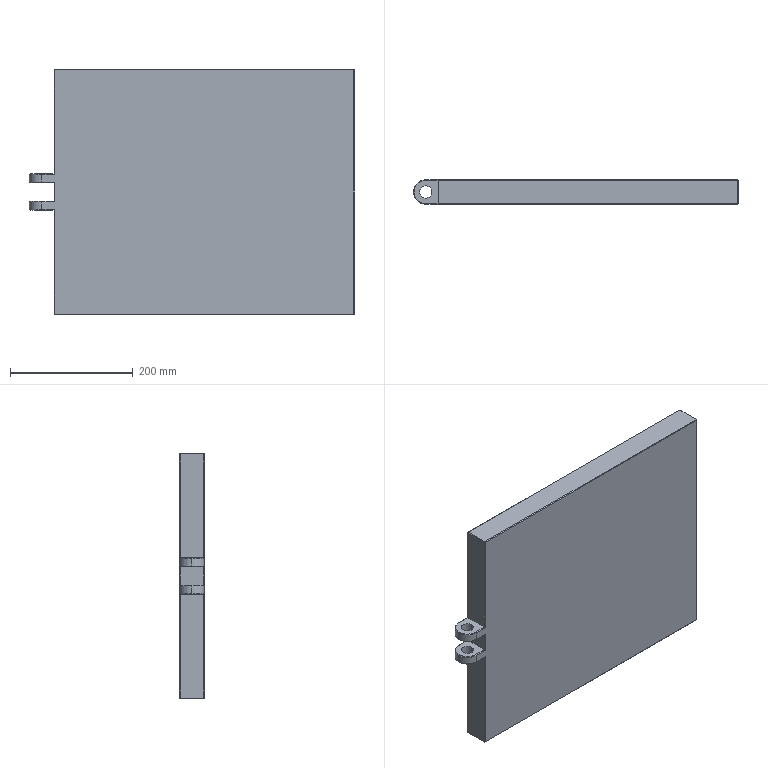Part | SolidWorks | 1 solid | 58 faces | box 530 x 40 x 400 mm | volume 7871394 mm3 | plane 44 | cylinder 8 | cone 6 | commonest cylinder face diameters 20 x4 40 x4
STEP:
#1=CARTESIAN_POINT('',(-284.,20.,30.));
#2=VERTEX_POINT('',#1);
#3=CARTESIAN_POINT('',(-265.,1.,30.));
#4=VERTEX_POINT('',#3);
#5=CARTESIAN_POINT('',(-265.,20.,30.));
#6=DIRECTION('',(0.,0.,1.));
#7=DIRECTION('',(1.,0.,0.));
#8=AXIS2_PLACEMENT_3D('',#5,#6,#7);
#9=CIRCLE('',#8,19.);
#10=EDGE_CURVE('',#2,#4,#9,.T.);
#11=ORIENTED_EDGE('',*,*,#10,.F.);
#12=CARTESIAN_POINT('',(-285.,20.,29.));
#13=VERTEX_POINT('',#12);
#14=CARTESIAN_POINT('',(-284.,20.,30.));
#15=DIRECTION('',(-0.7071,0.,-0.7071));
#16=VECTOR('',#15,1000.);
#17=LINE('',#14,#16);
#18=EDGE_CURVE('',#2,#13,#17,.T.);
#19=ORIENTED_EDGE('',*,*,#18,.T.);
#20=CARTESIAN_POINT('',(-265.,0.,29.));
#21=VERTEX_POINT('',#20);
#22=CARTESIAN_POINT('',(-265.,20.,29.));
#23=DIRECTION('',(0.,0.,-1.));
#24=DIRECTION('',(1.,0.,0.));
#25=AXIS2_PLACEMENT_3D('',#22,#23,#24);
#26=CIRCLE('',#25,20.);
#27=EDGE_CURVE('',#21,#13,#26,.T.);
#28=ORIENTED_EDGE('',*,*,#27,.F.);
#29=CARTESIAN_POINT('',(-265.,1.,30.));
#30=DIRECTION('',(0.,-0.7071,-0.7071));
#31=VECTOR('',#30,1000.);
#32=LINE('',#29,#31);
#33=EDGE_CURVE('',#4,#21,#32,.T.);
#34=ORIENTED_EDGE('',*,*,#33,.F.);
#35=EDGE_LOOP('',(#11,#19,#28,#34));
#36=FACE_OUTER_BOUND('',#35,.T.);
#37=CARTESIAN_POINT('',(-265.,20.,30.));
#38=DIRECTION('',(0.,0.,-1.));
#39=DIRECTION('',(-1.,0.,0.));
#40=AXIS2_PLACEMENT_3D('',#37,#38,#39);
#41=CONICAL_SURFACE('',#40,19.,0.7854);
#42=ADVANCED_FACE('',(#36),#41,.T.);
#43=CARTESIAN_POINT('',(-284.,20.,-15.));
#44=VERTEX_POINT('',#43);
#45=CARTESIAN_POINT('',(-265.,1.,-15.));
#46=VERTEX_POINT('',#45);
#47=CARTESIAN_POINT('',(-265.,20.,-15.));
#48=DIRECTION('',(0.,0.,1.));
#49=DIRECTION('',(-1.,0.,0.));
#50=AXIS2_PLACEMENT_3D('',#47,#48,#49);
#51=CIRCLE('',#50,19.);
#52=EDGE_CURVE('',#44,#46,#51,.T.);
#53=ORIENTED_EDGE('',*,*,#52,.F.);
#54=CARTESIAN_POINT('',(-285.,20.,-16.));
#55=VERTEX_POINT('',#54);
#56=CARTESIAN_POINT('',(-285.,20.,-16.));
#57=DIRECTION('',(-0.7071,0.,-0.7071));
#58=VECTOR('',#57,1000.);
#59=LINE('',#56,#58);
#60=EDGE_CURVE('',#44,#55,#59,.T.);
#61=ORIENTED_EDGE('',*,*,#60,.T.);
#62=CARTESIAN_POINT('',(-265.,0.,-16.));
#63=VERTEX_POINT('',#62);
#64=CARTESIAN_POINT('',(-265.,20.,-16.));
#65=DIRECTION('',(0.,0.,-1.));
#66=DIRECTION('',(-1.,0.,0.));
#67=AXIS2_PLACEMENT_3D('',#64,#65,#66);
#68=CIRCLE('',#67,20.);
#69=EDGE_CURVE('',#63,#55,#68,.T.);
#70=ORIENTED_EDGE('',*,*,#69,.F.);
#71=CARTESIAN_POINT('',(-265.,1.,-15.));
#72=DIRECTION('',(0.,-0.7071,-0.7071));
#73=VECTOR('',#72,1000.);
#74=LINE('',#71,#73);
#75=EDGE_CURVE('',#46,#63,#74,.T.);
#76=ORIENTED_EDGE('',*,*,#75,.F.);
#77=EDGE_LOOP('',(#53,#61,#70,#76));
#78=FACE_OUTER_BOUND('',#77,.T.);
#79=CARTESIAN_POINT('',(-265.,20.,-16.));
#80=DIRECTION('',(0.,0.,-1.));
#81=DIRECTION('',(-1.,0.,0.));
#82=AXIS2_PLACEMENT_3D('',#79,#80,#81);
#83=CONICAL_SURFACE('',#82,20.,0.7854);
#84=ADVANCED_FACE('',(#78),#83,.T.);
#85=CARTESIAN_POINT('',(-275.,20.,-30.));
#86=VERTEX_POINT('',#85);
#87=CARTESIAN_POINT('',(-255.,20.,-30.));
#88=VERTEX_POINT('',#87);
#89=CARTESIAN_POINT('',(-265.,20.,-30.));
#90=DIRECTION('',(0.,0.,1.));
#91=DIRECTION('',(1.,0.,0.));
#92=AXIS2_PLACEMENT_3D('',#89,#90,#91);
#93=CIRCLE('',#92,10.);
#94=EDGE_CURVE('',#86,#88,#93,.T.);
#95=ORIENTED_EDGE('',*,*,#94,.F.);
#96=CARTESIAN_POINT('',(-275.,20.,-15.));
#97=VERTEX_POINT('',#96);
#98=CARTESIAN_POINT('',(-275.,20.,-30.));
#99=DIRECTION('',(0.,0.,1.));
#100=VECTOR('',#99,1000.);
#101=LINE('',#98,#100);
#102=EDGE_CURVE('',#86,#97,#101,.T.);
#103=ORIENTED_EDGE('',*,*,#102,.T.);
#104=CARTESIAN_POINT('',(-255.,20.,-15.));
#105=VERTEX_POINT('',#104);
#106=CARTESIAN_POINT('',(-265.,20.,-15.));
#107=DIRECTION('',(0.,0.,1.));
#108=DIRECTION('',(-1.,0.,0.));
#109=AXIS2_PLACEMENT_3D('',#106,#107,#108);
#110=CIRCLE('',#109,10.);
#111=EDGE_CURVE('',#97,#105,#110,.T.);
#112=ORIENTED_EDGE('',*,*,#111,.T.);
#113=CARTESIAN_POINT('',(-255.,20.,-30.));
#114=DIRECTION('',(0.,0.,1.));
#115=VECTOR('',#114,1000.);
#116=LINE('',#113,#115);
#117=EDGE_CURVE('',#88,#105,#116,.T.);
#118=ORIENTED_EDGE('',*,*,#117,.F.);
#119=EDGE_LOOP('',(#95,#103,#112,#118));
#120=FACE_OUTER_BOUND('',#119,.T.);
#121=CARTESIAN_POINT('',(-265.,20.,-30.));
#122=DIRECTION('',(0.,0.,1.));
#123=DIRECTION('',(1.,0.,0.));
#124=AXIS2_PLACEMENT_3D('',#121,#122,#123);
#125=CYLINDRICAL_SURFACE('',#124,10.);
#126=ADVANCED_FACE('',(#120),#125,.F.);
#127=ORIENTED_EDGE('',*,*,#69,.T.);
#128=CARTESIAN_POINT('',(-285.,20.,-29.));
#129=VERTEX_POINT('',#128);
#130=CARTESIAN_POINT('',(-285.,20.,30.));
#131=DIRECTION('',(0.,0.,-1.));
#132=VECTOR('',#131,1000.);
#133=LINE('',#130,#132);
#134=EDGE_CURVE('',#55,#129,#133,.T.);
#135=ORIENTED_EDGE('',*,*,#134,.T.);
#136=CARTESIAN_POINT('',(-265.,0.,-29.));
#137=VERTEX_POINT('',#136);
#138=CARTESIAN_POINT('',(-265.,20.,-29.));
#139=DIRECTION('',(0.,0.,1.));
#140=DIRECTION('',(1.,0.,0.));
#141=AXIS2_PLACEMENT_3D('',#138,#139,#140);
#142=CIRCLE('',#141,20.);
#143=EDGE_CURVE('',#129,#137,#142,.T.);
#144=ORIENTED_EDGE('',*,*,#143,.T.);
#145=CARTESIAN_POINT('',(-265.,0.,30.));
#146=DIRECTION('',(0.,0.,-1.));
#147=VECTOR('',#146,1000.);
#148=LINE('',#145,#147);
#149=EDGE_CURVE('',#63,#137,#148,.T.);
#150=ORIENTED_EDGE('',*,*,#149,.F.);
#151=EDGE_LOOP('',(#127,#135,#144,#150));
#152=FACE_OUTER_BOUND('',#151,.T.);
#153=CARTESIAN_POINT('',(-265.,20.,30.));
#154=DIRECTION('',(0.,0.,-1.));
#155=DIRECTION('',(-1.,0.,0.));
#156=AXIS2_PLACEMENT_3D('',#153,#154,#155);
#157=CYLINDRICAL_SURFACE('',#156,20.);
#158=ADVANCED_FACE('',(#152),#157,.T.);
#159=CARTESIAN_POINT('',(-275.,20.,15.));
#160=VERTEX_POINT('',#159);
#161=CARTESIAN_POINT('',(-255.,20.,15.));
#162=VERTEX_POINT('',#161);
#163=CARTESIAN_POINT('',(-265.,20.,15.));
#164=DIRECTION('',(0.,0.,1.));
#165=DIRECTION('',(-1.,0.,0.));
#166=AXIS2_PLACEMENT_3D('',#163,#164,#165);
#167=CIRCLE('',#166,10.);
#168=EDGE_CURVE('',#160,#162,#167,.T.);
#169=ORIENTED_EDGE('',*,*,#168,.F.);
#170=CARTESIAN_POINT('',(-275.,20.,30.));
#171=VERTEX_POINT('',#170);
#172=CARTESIAN_POINT('',(-275.,20.,-30.));
#173=DIRECTION('',(0.,0.,1.));
#174=VECTOR('',#173,1000.);
#175=LINE('',#172,#174);
#176=EDGE_CURVE('',#160,#171,#175,.T.);
#177=ORIENTED_EDGE('',*,*,#176,.T.);
#178=CARTESIAN_POINT('',(-255.,20.,30.));
#179=VERTEX_POINT('',#178);
#180=CARTESIAN_POINT('',(-265.,20.,30.));
#181=DIRECTION('',(0.,0.,1.));
#182=DIRECTION('',(1.,0.,0.));
#183=AXIS2_PLACEMENT_3D('',#180,#181,#182);
#184=CIRCLE('',#183,10.);
#185=EDGE_CURVE('',#171,#179,#184,.T.);
#186=ORIENTED_EDGE('',*,*,#185,.T.);
#187=CARTESIAN_POINT('',(-255.,20.,-30.));
#188=DIRECTION('',(0.,0.,1.));
#189=VECTOR('',#188,1000.);
#190=LINE('',#187,#189);
#191=EDGE_CURVE('',#162,#179,#190,.T.);
#192=ORIENTED_EDGE('',*,*,#191,.F.);
#193=EDGE_LOOP('',(#169,#177,#186,#192));
#194=FACE_OUTER_BOUND('',#193,.T.);
#195=CARTESIAN_POINT('',(-265.,20.,-30.));
#196=DIRECTION('',(0.,0.,1.));
#197=DIRECTION('',(1.,0.,0.));
#198=AXIS2_PLACEMENT_3D('',#195,#196,#197);
#199=CYLINDRICAL_SURFACE('',#198,10.);
#200=ADVANCED_FACE('',(#194),#199,.F.);
#201=ORIENTED_EDGE('',*,*,#27,.T.);
#202=CARTESIAN_POINT('',(-285.,20.,16.));
#203=VERTEX_POINT('',#202);
#204=CARTESIAN_POINT('',(-285.,20.,30.));
#205=DIRECTION('',(0.,0.,-1.));
#206=VECTOR('',#205,1000.);
#207=LINE('',#204,#206);
#208=EDGE_CURVE('',#13,#203,#207,.T.);
#209=ORIENTED_EDGE('',*,*,#208,.T.);
#210=CARTESIAN_POINT('',(-265.,0.,16.));
#211=VERTEX_POINT('',#210);
#212=CARTESIAN_POINT('',(-265.,20.,16.));
#213=DIRECTION('',(0.,0.,1.));
#214=DIRECTION('',(-1.,0.,0.));
#215=AXIS2_PLACEMENT_3D('',#212,#213,#214);
#216=CIRCLE('',#215,20.);
#217=EDGE_CURVE('',#203,#211,#216,.T.);
#218=ORIENTED_EDGE('',*,*,#217,.T.);
#219=CARTESIAN_POINT('',(-265.,0.,30.));
#220=DIRECTION('',(0.,0.,-1.));
#221=VECTOR('',#220,1000.);
#222=LINE('',#219,#221);
#223=EDGE_CURVE('',#21,#211,#222,.T.);
#224=ORIENTED_EDGE('',*,*,#223,.F.);
#225=EDGE_LOOP('',(#201,#209,#218,#224));
#226=FACE_OUTER_BOUND('',#225,.T.);
#227=CARTESIAN_POINT('',(-265.,20.,30.));
#228=DIRECTION('',(0.,0.,-1.));
#229=DIRECTION('',(-1.,0.,0.));
#230=AXIS2_PLACEMENT_3D('',#227,#228,#229);
#231=CYLINDRICAL_SURFACE('',#230,20.);
#232=ADVANCED_FACE('',(#226),#231,.T.);
#233=ORIENTED_EDGE('',*,*,#208,.F.);
#234=CARTESIAN_POINT('',(-265.,40.,29.));
#235=VERTEX_POINT('',#234);
#236=CARTESIAN_POINT('',(-265.,20.,29.));
#237=DIRECTION('',(0.,0.,-1.));
#238=DIRECTION('',(1.,0.,0.));
#239=AXIS2_PLACEMENT_3D('',#236,#237,#238);
#240=CIRCLE('',#239,20.);
#241=EDGE_CURVE('',#13,#235,#240,.T.);
#242=ORIENTED_EDGE('',*,*,#241,.T.);
#243=CARTESIAN_POINT('',(-265.,40.,16.));
#244=VERTEX_POINT('',#243);
#245=CARTESIAN_POINT('',(-265.,40.,30.));
#246=DIRECTION('',(0.,0.,-1.));
#247=VECTOR('',#246,1000.);
#248=LINE('',#245,#247);
#249=EDGE_CURVE('',#235,#244,#248,.T.);
#250=ORIENTED_EDGE('',*,*,#249,.T.);
#251=CARTESIAN_POINT('',(-265.,20.,16.));
#252=DIRECTION('',(0.,0.,1.));
#253=DIRECTION('',(-1.,0.,0.));
#254=AXIS2_PLACEMENT_3D('',#251,#252,#253);
#255=CIRCLE('',#254,20.);
#256=EDGE_CURVE('',#244,#203,#255,.T.);
#257=ORIENTED_EDGE('',*,*,#256,.T.);
#258=EDGE_LOOP('',(#233,#242,#250,#257));
#259=FACE_OUTER_BOUND('',#258,.T.);
#260=CARTESIAN_POINT('',(-265.,20.,30.));
#261=DIRECTION('',(0.,0.,-1.));
#262=DIRECTION('',(-1.,0.,0.));
#263=AXIS2_PLACEMENT_3D('',#260,#261,#262);
#264=CYLINDRICAL_SURFACE('',#263,20.);
#265=ADVANCED_FACE('',(#259),#264,.T.);
#266=ORIENTED_EDGE('',*,*,#176,.F.);
#267=CARTESIAN_POINT('',(-265.,20.,15.));
#268=DIRECTION('',(0.,0.,1.));
#269=DIRECTION('',(-1.,0.,0.));
#270=AXIS2_PLACEMENT_3D('',#267,#268,#269);
#271=CIRCLE('',#270,10.);
#272=EDGE_CURVE('',#162,#160,#271,.T.);
#273=ORIENTED_EDGE('',*,*,#272,.F.);
#274=ORIENTED_EDGE('',*,*,#191,.T.);
#275=CARTESIAN_POINT('',(-265.,20.,30.));
#276=DIRECTION('',(0.,0.,1.));
#277=DIRECTION('',(1.,0.,0.));
#278=AXIS2_PLACEMENT_3D('',#275,#276,#277);
#279=CIRCLE('',#278,10.);
#280=EDGE_CURVE('',#179,#171,#279,.T.);
#281=ORIENTED_EDGE('',*,*,#280,.T.);
#282=EDGE_LOOP('',(#266,#273,#274,#281));
#283=FACE_OUTER_BOUND('',#282,.T.);
#284=CARTESIAN_POINT('',(-265.,20.,-30.));
#285=DIRECTION('',(0.,0.,1.));
#286=DIRECTION('',(1.,0.,0.));
#287=AXIS2_PLACEMENT_3D('',#284,#285,#286);
#288=CYLINDRICAL_SURFACE('',#287,10.);
#289=ADVANCED_FACE('',(#283),#288,.F.);
#290=CARTESIAN_POINT('',(-245.,39.,-199.));
#291=VERTEX_POINT('',#290);
#292=CARTESIAN_POINT('',(-245.,1.,-199.));
#293=VERTEX_POINT('',#292);
#294=CARTESIAN_POINT('',(-245.,40.,-199.));
#295=DIRECTION('',(0.,-1.,0.));
#296=VECTOR('',#295,1000.);
#297=LINE('',#294,#296);
#298=EDGE_CURVE('',#291,#293,#297,.T.);
#299=ORIENTED_EDGE('',*,*,#298,.T.);
#300=CARTESIAN_POINT('',(-245.,1.,-30.));
#301=VERTEX_POINT('',#300);
#302=CARTESIAN_POINT('',(-245.,1.,-200.));
#303=DIRECTION('',(0.,0.,1.));
#304=VECTOR('',#303,1000.);
#305=LINE('',#302,#304);
#306=EDGE_CURVE('',#293,#301,#305,.T.);
#307=ORIENTED_EDGE('',*,*,#306,.T.);
#308=CARTESIAN_POINT('',(-245.,39.,-30.));
#309=VERTEX_POINT('',#308);
#310=CARTESIAN_POINT('',(-245.,40.,-30.));
#311=DIRECTION('',(0.,-1.,0.));
#312=VECTOR('',#311,1000.);
#313=LINE('',#310,#312);
#314=EDGE_CURVE('',#309,#301,#313,.T.);
#315=ORIENTED_EDGE('',*,*,#314,.F.);
#316=CARTESIAN_POINT('',(-245.,39.,-200.));
#317=DIRECTION('',(0.,0.,-1.));
#318=VECTOR('',#317,1000.);
#319=LINE('',#316,#318);
#320=EDGE_CURVE('',#309,#291,#319,.T.);
#321=ORIENTED_EDGE('',*,*,#320,.T.);
#322=EDGE_LOOP('',(#299,#307,#315,#321));
#323=FACE_OUTER_BOUND('',#322,.T.);
#324=CARTESIAN_POINT('',(-245.,40.,-200.));
#325=DIRECTION('',(1.,0.,0.));
#326=DIRECTION('',(0.,0.,-1.));
#327=AXIS2_PLACEMENT_3D('',#324,#325,#326);
#328=PLANE('',#327);
#329=ADVANCED_FACE('',(#323),#328,.F.);
#330=CARTESIAN_POINT('',(245.,1.,199.));
#331=VERTEX_POINT('',#330);
#332=CARTESIAN_POINT('',(245.,1.,-199.));
#333=VERTEX_POINT('',#332);
#334=CARTESIAN_POINT('',(245.,1.,-200.));
#335=DIRECTION('',(0.,0.,-1.));
#336=VECTOR('',#335,1000.);
#337=LINE('',#334,#336);
#338=EDGE_CURVE('',#331,#333,#337,.T.);
#339=ORIENTED_EDGE('',*,*,#338,.T.);
#340=CARTESIAN_POINT('',(245.,39.,-199.));
#341=VERTEX_POINT('',#340);
#342=CARTESIAN_POINT('',(245.,40.,-199.));
#343=DIRECTION('',(0.,1.,0.));
#344=VECTOR('',#343,1000.);
#345=LINE('',#342,#344);
#346=EDGE_CURVE('',#333,#341,#345,.T.);
#347=ORIENTED_EDGE('',*,*,#346,.T.);
#348=CARTESIAN_POINT('',(245.,39.,199.));
#349=VERTEX_POINT('',#348);
#350=CARTESIAN_POINT('',(245.,39.,200.));
#351=DIRECTION('',(0.,0.,1.));
#352=VECTOR('',#351,1000.);
#353=LINE('',#350,#352);
#354=EDGE_CURVE('',#341,#349,#353,.T.);
#355=ORIENTED_EDGE('',*,*,#354,.T.);
#356=CARTESIAN_POINT('',(245.,40.,199.));
#357=DIRECTION('',(0.,-1.,0.));
#358=VECTOR('',#357,1000.);
#359=LINE('',#356,#358);
#360=EDGE_CURVE('',#349,#331,#359,.T.);
#361=ORIENTED_EDGE('',*,*,#360,.T.);
#362=EDGE_LOOP('',(#339,#347,#355,#361));
#363=FACE_OUTER_BOUND('',#362,.T.);
#364=CARTESIAN_POINT('',(245.,40.,-200.));
#365=DIRECTION('',(-1.,0.,0.));
#366=DIRECTION('',(0.,0.,1.));
#367=AXIS2_PLACEMENT_3D('',#364,#365,#366);
#368=PLANE('',#367);
#369=ADVANCED_FACE('',(#363),#368,.F.);
#370=CARTESIAN_POINT('',(244.,39.,-200.));
#371=VERTEX_POINT('',#370);
#372=CARTESIAN_POINT('',(244.,1.,-200.));
#373=VERTEX_POINT('',#372);
#374=CARTESIAN_POINT('',(244.,40.,-200.));
#375=DIRECTION('',(0.,-1.,0.));
#376=VECTOR('',#375,1000.);
#377=LINE('',#374,#376);
#378=EDGE_CURVE('',#371,#373,#377,.T.);
#379=ORIENTED_EDGE('',*,*,#378,.T.);
#380=CARTESIAN_POINT('',(-244.,1.,-200.));
#381=VERTEX_POINT('',#380);
#382=CARTESIAN_POINT('',(-245.,1.,-200.));
#383=DIRECTION('',(-1.,0.,0.));
#384=VECTOR('',#383,1000.);
#385=LINE('',#382,#384);
#386=EDGE_CURVE('',#373,#381,#385,.T.);
#387=ORIENTED_EDGE('',*,*,#386,.T.);
#388=CARTESIAN_POINT('',(-244.,39.,-200.));
#389=VERTEX_POINT('',#388);
#390=CARTESIAN_POINT('',(-244.,40.,-200.));
#391=DIRECTION('',(0.,1.,0.));
#392=VECTOR('',#391,1000.);
#393=LINE('',#390,#392);
#394=EDGE_CURVE('',#381,#389,#393,.T.);
#395=ORIENTED_EDGE('',*,*,#394,.T.);
#396=CARTESIAN_POINT('',(245.,39.,-200.));
#397=DIRECTION('',(1.,0.,0.));
#398=VECTOR('',#397,1000.);
#399=LINE('',#396,#398);
#400=EDGE_CURVE('',#389,#371,#399,.T.);
#401=ORIENTED_EDGE('',*,*,#400,.T.);
#402=EDGE_LOOP('',(#379,#387,#395,#401));
#403=FACE_OUTER_BOUND('',#402,.T.);
#404=CARTESIAN_POINT('',(-245.,40.,-200.));
#405=DIRECTION('',(0.,0.,1.));
#406=DIRECTION('',(1.,0.,0.));
#407=AXIS2_PLACEMENT_3D('',#404,#405,#406);
#408=PLANE('',#407);
#409=ADVANCED_FACE('',(#403),#408,.F.);
#410=CARTESIAN_POINT('',(-245.,39.,30.));
#411=VERTEX_POINT('',#410);
#412=CARTESIAN_POINT('',(-245.,1.,30.));
#413=VERTEX_POINT('',#412);
#414=CARTESIAN_POINT('',(-245.,40.,30.));
#415=DIRECTION('',(0.,-1.,0.));
#416=VECTOR('',#415,1000.);
#417=LINE('',#414,#416);
#418=EDGE_CURVE('',#411,#413,#417,.T.);
#419=ORIENTED_EDGE('',*,*,#418,.T.);
#420=CARTESIAN_POINT('',(-245.,1.,199.));
#421=VERTEX_POINT('',#420);
#422=CARTESIAN_POINT('',(-245.,1.,-200.));
#423=DIRECTION('',(0.,0.,1.));
#424=VECTOR('',#423,1000.);
#425=LINE('',#422,#424);
#426=EDGE_CURVE('',#413,#421,#425,.T.);
#427=ORIENTED_EDGE('',*,*,#426,.T.);
#428=CARTESIAN_POINT('',(-245.,39.,199.));
#429=VERTEX_POINT('',#428);
#430=CARTESIAN_POINT('',(-245.,40.,199.));
#431=DIRECTION('',(0.,1.,0.));
#432=VECTOR('',#431,1000.);
#433=LINE('',#430,#432);
#434=EDGE_CURVE('',#421,#429,#433,.T.);
#435=ORIENTED_EDGE('',*,*,#434,.T.);
#436=CARTESIAN_POINT('',(-245.,39.,30.));
#437=DIRECTION('',(0.,0.,-1.));
#438=VECTOR('',#437,1000.);
#439=LINE('',#436,#438);
#440=EDGE_CURVE('',#429,#411,#439,.T.);
#441=ORIENTED_EDGE('',*,*,#440,.T.);
#442=EDGE_LOOP('',(#419,#427,#435,#441));
#443=FACE_OUTER_BOUND('',#442,.T.);
#444=CARTESIAN_POINT('',(-245.,40.,-200.));
#445=DIRECTION('',(1.,0.,0.));
#446=DIRECTION('',(0.,0.,-1.));
#447=AXIS2_PLACEMENT_3D('',#444,#445,#446);
#448=PLANE('',#447);
#449=ADVANCED_FACE('',(#443),#448,.F.);
#450=CARTESIAN_POINT('',(244.,39.,200.));
#451=VERTEX_POINT('',#450);
#452=CARTESIAN_POINT('',(-244.,39.,200.));
#453=VERTEX_POINT('',#452);
#454=CARTESIAN_POINT('',(-245.,39.,200.));
#455=DIRECTION('',(-1.,0.,0.));
#456=VECTOR('',#455,1000.);
#457=LINE('',#454,#456);
#458=EDGE_CURVE('',#451,#453,#457,.T.);
#459=ORIENTED_EDGE('',*,*,#458,.T.);
#460=CARTESIAN_POINT('',(-244.,1.,200.));
#461=VERTEX_POINT('',#460);
#462=CARTESIAN_POINT('',(-244.,40.,200.));
#463=DIRECTION('',(0.,-1.,0.));
#464=VECTOR('',#463,1000.);
#465=LINE('',#462,#464);
#466=EDGE_CURVE('',#453,#461,#465,.T.);
#467=ORIENTED_EDGE('',*,*,#466,.T.);
#468=CARTESIAN_POINT('',(244.,1.,200.));
#469=VERTEX_POINT('',#468);
#470=CARTESIAN_POINT('',(-245.,1.,200.));
#471=DIRECTION('',(1.,0.,0.));
#472=VECTOR('',#471,1000.);
#473=LINE('',#470,#472);
#474=EDGE_CURVE('',#461,#469,#473,.T.);
#475=ORIENTED_EDGE('',*,*,#474,.T.);
#476=CARTESIAN_POINT('',(244.,40.,200.));
#477=DIRECTION('',(0.,1.,0.));
#478=VECTOR('',#477,1000.);
#479=LINE('',#476,#478);
#480=EDGE_CURVE('',#469,#451,#479,.T.);
#481=ORIENTED_EDGE('',*,*,#480,.T.);
#482=EDGE_LOOP('',(#459,#467,#475,#481));
#483=FACE_OUTER_BOUND('',#482,.T.);
#484=CARTESIAN_POINT('',(-245.,40.,200.));
#485=DIRECTION('',(0.,0.,-1.));
#486=DIRECTION('',(-1.,0.,0.));
#487=AXIS2_PLACEMENT_3D('',#484,#485,#486);
#488=PLANE('',#487);
#489=ADVANCED_FACE('',(#483),#488,.F.);
#490=CARTESIAN_POINT('',(-244.,40.,-199.));
#491=VERTEX_POINT('',#490);
#492=CARTESIAN_POINT('',(-244.,40.,-29.));
#493=VERTEX_POINT('',#492);
#494=CARTESIAN_POINT('',(-244.,40.,-30.));
#495=DIRECTION('',(0.,0.,1.));
#496=VECTOR('',#495,1000.);
#497=LINE('',#494,#496);
#498=EDGE_CURVE('',#491,#493,#497,.T.);
#499=ORIENTED_EDGE('',*,*,#498,.T.);
#500=CARTESIAN_POINT('',(-265.,40.,-29.));
#501=VERTEX_POINT('',#500);
#502=CARTESIAN_POINT('',(-265.,40.,-29.));
#503=DIRECTION('',(-1.,0.,0.));
#504=VECTOR('',#503,1000.);
#505=LINE('',#502,#504);
#506=EDGE_CURVE('',#493,#501,#505,.T.);
#507=ORIENTED_EDGE('',*,*,#506,.T.);
#508=CARTESIAN_POINT('',(-265.,40.,-16.));
#509=VERTEX_POINT('',#508);
#510=CARTESIAN_POINT('',(-265.,40.,30.));
#511=DIRECTION('',(0.,0.,-1.));
#512=VECTOR('',#511,1000.);
#513=LINE('',#510,#512);
#514=EDGE_CURVE('',#509,#501,#513,.T.);
#515=ORIENTED_EDGE('',*,*,#514,.F.);
#516=CARTESIAN_POINT('',(-244.,40.,-16.));
#517=VERTEX_POINT('',#516);
#518=CARTESIAN_POINT('',(-245.,40.,-16.));
#519=DIRECTION('',(1.,0.,0.));
#520=VECTOR('',#519,1000.);
#521=LINE('',#518,#520);
#522=EDGE_CURVE('',#509,#517,#521,.T.);
#523=ORIENTED_EDGE('',*,*,#522,.T.);
#524=CARTESIAN_POINT('',(-244.,40.,16.));
#525=VERTEX_POINT('',#524);
#526=CARTESIAN_POINT('',(-244.,40.,15.));
#527=DIRECTION('',(0.,0.,1.));
#528=VECTOR('',#527,1000.);
#529=LINE('',#526,#528);
#530=EDGE_CURVE('',#517,#525,#529,.T.);
#531=ORIENTED_EDGE('',*,*,#530,.T.);
#532=CARTESIAN_POINT('',(0.,40.,16.));
#533=DIRECTION('',(-1.,0.,0.));
#534=VECTOR('',#533,1000.);
#535=LINE('',#532,#534);
#536=EDGE_CURVE('',#525,#244,#535,.T.);
#537=ORIENTED_EDGE('',*,*,#536,.T.);
#538=ORIENTED_EDGE('',*,*,#249,.F.);
#539=CARTESIAN_POINT('',(-244.,40.,29.));
#540=VERTEX_POINT('',#539);
#541=CARTESIAN_POINT('',(0.,40.,29.));
#542=DIRECTION('',(1.,0.,0.));
#543=VECTOR('',#542,1000.);
#544=LINE('',#541,#543);
#545=EDGE_CURVE('',#235,#540,#544,.T.);
#546=ORIENTED_EDGE('',*,*,#545,.T.);
#547=CARTESIAN_POINT('',(-244.,40.,199.));
#548=VERTEX_POINT('',#547);
#549=CARTESIAN_POINT('',(-244.,40.,200.));
#550=DIRECTION('',(0.,0.,1.));
#551=VECTOR('',#550,1000.);
#552=LINE('',#549,#551);
#553=EDGE_CURVE('',#540,#548,#552,.T.);
#554=ORIENTED_EDGE('',*,*,#553,.T.);
#555=CARTESIAN_POINT('',(244.,40.,199.));
#556=VERTEX_POINT('',#555);
#557=CARTESIAN_POINT('',(245.,40.,199.));
#558=DIRECTION('',(1.,0.,0.));
#559=VECTOR('',#558,1000.);
#560=LINE('',#557,#559);
#561=EDGE_CURVE('',#548,#556,#560,.T.);
#562=ORIENTED_EDGE('',*,*,#561,.T.);
#563=CARTESIAN_POINT('',(244.,40.,-199.));
#564=VERTEX_POINT('',#563);
#565=CARTESIAN_POINT('',(244.,40.,-200.));
#566=DIRECTION('',(0.,0.,-1.));
#567=VECTOR('',#566,1000.);
#568=LINE('',#565,#567);
#569=EDGE_CURVE('',#556,#564,#568,.T.);
#570=ORIENTED_EDGE('',*,*,#569,.T.);
#571=CARTESIAN_POINT('',(-245.,40.,-199.));
#572=DIRECTION('',(-1.,0.,0.));
#573=VECTOR('',#572,1000.);
#574=LINE('',#571,#573);
#575=EDGE_CURVE('',#564,#491,#574,.T.);
#576=ORIENTED_EDGE('',*,*,#575,.T.);
#577=EDGE_LOOP('',(#499,#507,#515,#523,#531,#537,#538,#546,#554,#562,#570,#576));
#578=FACE_OUTER_BOUND('',#577,.T.);
#579=CARTESIAN_POINT('',(0.,40.,0.));
#580=DIRECTION('',(0.,1.,0.));
#581=DIRECTION('',(0.,0.,1.));
#582=AXIS2_PLACEMENT_3D('',#579,#580,#581);
#583=PLANE('',#582);
#584=ADVANCED_FACE('',(#578),#583,.T.);
#585=ORIENTED_EDGE('',*,*,#223,.T.);
#586=CARTESIAN_POINT('',(-244.,0.,16.));
#587=VERTEX_POINT('',#586);
#588=CARTESIAN_POINT('',(-245.,0.,16.));
#589=DIRECTION('',(1.,0.,0.));
#590=VECTOR('',#589,1000.);
#591=LINE('',#588,#590);
#592=EDGE_CURVE('',#211,#587,#591,.T.);
#593=ORIENTED_EDGE('',*,*,#592,.T.);
#594=CARTESIAN_POINT('',(-244.,0.,-16.));
#595=VERTEX_POINT('',#594);
#596=CARTESIAN_POINT('',(-244.,0.,0.));
#597=DIRECTION('',(0.,0.,-1.));
#598=VECTOR('',#597,1000.);
#599=LINE('',#596,#598);
#600=EDGE_CURVE('',#587,#595,#599,.T.);
#601=ORIENTED_EDGE('',*,*,#600,.T.);
#602=CARTESIAN_POINT('',(0.,0.,-16.));
#603=DIRECTION('',(-1.,0.,0.));
#604=VECTOR('',#603,1000.);
#605=LINE('',#602,#604);
#606=EDGE_CURVE('',#595,#63,#605,.T.);
#607=ORIENTED_EDGE('',*,*,#606,.T.);
#608=ORIENTED_EDGE('',*,*,#149,.T.);
#609=CARTESIAN_POINT('',(-244.,0.,-29.));
#610=VERTEX_POINT('',#609);
#611=CARTESIAN_POINT('',(0.,0.,-29.));
#612=DIRECTION('',(1.,0.,0.));
#613=VECTOR('',#612,1000.);
#614=LINE('',#611,#613);
#615=EDGE_CURVE('',#137,#610,#614,.T.);
#616=ORIENTED_EDGE('',*,*,#615,.T.);
#617=CARTESIAN_POINT('',(-244.,0.,-199.));
#618=VERTEX_POINT('',#617);
#619=CARTESIAN_POINT('',(-244.,0.,0.));
#620=DIRECTION('',(0.,0.,-1.));
#621=VECTOR('',#620,1000.);
#622=LINE('',#619,#621);
#623=EDGE_CURVE('',#610,#618,#622,.T.);
#624=ORIENTED_EDGE('',*,*,#623,.T.);
#625=CARTESIAN_POINT('',(244.,0.,-199.));
#626=VERTEX_POINT('',#625);
#627=CARTESIAN_POINT('',(0.,0.,-199.));
#628=DIRECTION('',(1.,0.,0.));
#629=VECTOR('',#628,1000.);
#630=LINE('',#627,#629);
#631=EDGE_CURVE('',#618,#626,#630,.T.);
#632=ORIENTED_EDGE('',*,*,#631,.T.);
#633=CARTESIAN_POINT('',(244.,0.,199.));
#634=VERTEX_POINT('',#633);
#635=CARTESIAN_POINT('',(244.,0.,0.));
#636=DIRECTION('',(0.,0.,1.));
#637=VECTOR('',#636,1000.);
#638=LINE('',#635,#637);
#639=EDGE_CURVE('',#626,#634,#638,.T.);
#640=ORIENTED_EDGE('',*,*,#639,.T.);
#641=CARTESIAN_POINT('',(-244.,0.,199.));
#642=VERTEX_POINT('',#641);
#643=CARTESIAN_POINT('',(0.,0.,199.));
#644=DIRECTION('',(-1.,0.,0.));
#645=VECTOR('',#644,1000.);
#646=LINE('',#643,#645);
#647=EDGE_CURVE('',#634,#642,#646,.T.);
#648=ORIENTED_EDGE('',*,*,#647,.T.);
#649=CARTESIAN_POINT('',(-244.,0.,29.));
#650=VERTEX_POINT('',#649);
#651=CARTESIAN_POINT('',(-244.,0.,0.));
#652=DIRECTION('',(0.,0.,-1.));
#653=VECTOR('',#652,1000.);
#654=LINE('',#651,#653);
#655=EDGE_CURVE('',#642,#650,#654,.T.);
#656=ORIENTED_EDGE('',*,*,#655,.T.);
#657=CARTESIAN_POINT('',(-265.,0.,29.));
#658=DIRECTION('',(-1.,0.,0.));
#659=VECTOR('',#658,1000.);
#660=LINE('',#657,#659);
#661=EDGE_CURVE('',#650,#21,#660,.T.);
#662=ORIENTED_EDGE('',*,*,#661,.T.);
#663=EDGE_LOOP('',(#585,#593,#601,#607,#608,#616,#624,#632,#640,#648,#656,#662));
#664=FACE_OUTER_BOUND('',#663,.T.);
#665=CARTESIAN_POINT('',(0.,0.,0.));
#666=DIRECTION('',(0.,1.,0.));
#667=DIRECTION('',(0.,0.,1.));
#668=AXIS2_PLACEMENT_3D('',#665,#666,#667);
#669=PLANE('',#668);
#670=ADVANCED_FACE('',(#664),#669,.F.);
#671=ORIENTED_EDGE('',*,*,#280,.F.);
#672=ORIENTED_EDGE('',*,*,#185,.F.);
#673=EDGE_LOOP('',(#671,#672));
#674=FACE_BOUND('',#673,.T.);
#675=CARTESIAN_POINT('',(-265.,39.,30.));
#676=VERTEX_POINT('',#675);
#677=CARTESIAN_POINT('',(-265.,20.,30.));
#678=DIRECTION('',(0.,0.,1.));
#679=DIRECTION('',(1.,0.,0.));
#680=AXIS2_PLACEMENT_3D('',#677,#678,#679);
#681=CIRCLE('',#680,19.);
#682=EDGE_CURVE('',#676,#2,#681,.T.);
#683=ORIENTED_EDGE('',*,*,#682,.T.);
#684=ORIENTED_EDGE('',*,*,#10,.T.);
#685=CARTESIAN_POINT('',(-245.,1.,30.));
#686=DIRECTION('',(1.,0.,0.));
#687=VECTOR('',#686,1000.);
#688=LINE('',#685,#687);
#689=EDGE_CURVE('',#4,#413,#688,.T.);
#690=ORIENTED_EDGE('',*,*,#689,.T.);
#691=ORIENTED_EDGE('',*,*,#418,.F.);
#692=CARTESIAN_POINT('',(-223.563,39.,30.));
#693=DIRECTION('',(-1.,0.,0.));
#694=VECTOR('',#693,1000.);
#695=LINE('',#692,#694);
#696=EDGE_CURVE('',#411,#676,#695,.T.);
#697=ORIENTED_EDGE('',*,*,#696,.T.);
#698=EDGE_LOOP('',(#683,#684,#690,#691,#697));
#699=FACE_OUTER_BOUND('',#698,.T.);
#700=CARTESIAN_POINT('',(-223.563,20.,30.));
#701=DIRECTION('',(0.,0.,1.));
#702=DIRECTION('',(1.,0.,0.));
#703=AXIS2_PLACEMENT_3D('',#700,#701,#702);
#704=PLANE('',#703);
#705=ADVANCED_FACE('',(#674,#699),#704,.T.);
#706=CARTESIAN_POINT('',(-265.,20.,-30.));
#707=DIRECTION('',(0.,0.,1.));
#708=DIRECTION('',(1.,0.,0.));
#709=AXIS2_PLACEMENT_3D('',#706,#707,#708);
#710=CIRCLE('',#709,10.);
#711=EDGE_CURVE('',#88,#86,#710,.T.);
#712=ORIENTED_EDGE('',*,*,#711,.T.);
#713=ORIENTED_EDGE('',*,*,#94,.T.);
#714=EDGE_LOOP('',(#712,#713));
#715=FACE_BOUND('',#714,.T.);
#716=ORIENTED_EDGE('',*,*,#314,.T.);
#717=CARTESIAN_POINT('',(-265.,1.,-30.));
#718=VERTEX_POINT('',#717);
#719=CARTESIAN_POINT('',(-223.563,1.,-30.));
#720=DIRECTION('',(-1.,0.,0.));
#721=VECTOR('',#720,1000.);
#722=LINE('',#719,#721);
#723=EDGE_CURVE('',#301,#718,#722,.T.);
#724=ORIENTED_EDGE('',*,*,#723,.T.);
#725=CARTESIAN_POINT('',(-265.,39.,-30.));
#726=VERTEX_POINT('',#725);
#727=CARTESIAN_POINT('',(-265.,20.,-30.));
#728=DIRECTION('',(0.,0.,-1.));
#729=DIRECTION('',(1.,0.,0.));
#730=AXIS2_PLACEMENT_3D('',#727,#728,#729);
#731=CIRCLE('',#730,19.);
#732=EDGE_CURVE('',#718,#726,#731,.T.);
#733=ORIENTED_EDGE('',*,*,#732,.T.);
#734=CARTESIAN_POINT('',(-245.,39.,-30.));
#735=DIRECTION('',(1.,0.,0.));
#736=VECTOR('',#735,1000.);
#737=LINE('',#734,#736);
#738=EDGE_CURVE('',#726,#309,#737,.T.);
#739=ORIENTED_EDGE('',*,*,#738,.T.);
#740=EDGE_LOOP('',(#716,#724,#733,#739));
#741=FACE_OUTER_BOUND('',#740,.T.);
#742=CARTESIAN_POINT('',(-223.563,20.,-30.));
#743=DIRECTION('',(0.,0.,1.));
#744=DIRECTION('',(1.,0.,0.));
#745=AXIS2_PLACEMENT_3D('',#742,#743,#744);
#746=PLANE('',#745);
#747=ADVANCED_FACE('',(#715,#741),#746,.F.);
#748=ORIENTED_EDGE('',*,*,#134,.F.);
#749=CARTESIAN_POINT('',(-265.,20.,-16.));
#750=DIRECTION('',(0.,0.,-1.));
#751=DIRECTION('',(-1.,0.,0.));
#752=AXIS2_PLACEMENT_3D('',#749,#750,#751);
#753=CIRCLE('',#752,20.);
#754=EDGE_CURVE('',#55,#509,#753,.T.);
#755=ORIENTED_EDGE('',*,*,#754,.T.);
#756=ORIENTED_EDGE('',*,*,#514,.T.);
#757=CARTESIAN_POINT('',(-265.,20.,-29.));
#758=DIRECTION('',(0.,0.,1.));
#759=DIRECTION('',(1.,0.,0.));
#760=AXIS2_PLACEMENT_3D('',#757,#758,#759);
#761=CIRCLE('',#760,20.);
#762=EDGE_CURVE('',#501,#129,#761,.T.);
#763=ORIENTED_EDGE('',*,*,#762,.T.);
#764=EDGE_LOOP('',(#748,#755,#756,#763));
#765=FACE_OUTER_BOUND('',#764,.T.);
#766=CARTESIAN_POINT('',(-265.,20.,30.));
#767=DIRECTION('',(0.,0.,-1.));
#768=DIRECTION('',(-1.,0.,0.));
#769=AXIS2_PLACEMENT_3D('',#766,#767,#768);
#770=CYLINDRICAL_SURFACE('',#769,20.);
#771=ADVANCED_FACE('',(#765),#770,.T.);
#772=ORIENTED_EDGE('',*,*,#102,.F.);
#773=ORIENTED_EDGE('',*,*,#711,.F.);
#774=ORIENTED_EDGE('',*,*,#117,.T.);
#775=CARTESIAN_POINT('',(-265.,20.,-15.));
#776=DIRECTION('',(0.,0.,1.));
#777=DIRECTION('',(-1.,0.,0.));
#778=AXIS2_PLACEMENT_3D('',#775,#776,#777);
#779=CIRCLE('',#778,10.);
#780=EDGE_CURVE('',#105,#97,#779,.T.);
#781=ORIENTED_EDGE('',*,*,#780,.T.);
#782=EDGE_LOOP('',(#772,#773,#774,#781));
#783=FACE_OUTER_BOUND('',#782,.T.);
#784=CARTESIAN_POINT('',(-265.,20.,-30.));
#785=DIRECTION('',(0.,0.,1.));
#786=DIRECTION('',(1.,0.,0.));
#787=AXIS2_PLACEMENT_3D('',#784,#785,#786);
#788=CYLINDRICAL_SURFACE('',#787,10.);
#789=ADVANCED_FACE('',(#783),#788,.F.);
#790=CARTESIAN_POINT('',(-245.,1.,-15.));
#791=VERTEX_POINT('',#790);
#792=CARTESIAN_POINT('',(-245.,39.,-15.));
#793=VERTEX_POINT('',#792);
#794=CARTESIAN_POINT('',(-245.,40.,-15.));
#795=DIRECTION('',(0.,1.,0.));
#796=VECTOR('',#795,1000.);
#797=LINE('',#794,#796);
#798=EDGE_CURVE('',#791,#793,#797,.T.);
#799=ORIENTED_EDGE('',*,*,#798,.F.);
#800=CARTESIAN_POINT('',(-245.,1.,15.));
#801=VERTEX_POINT('',#800);
#802=CARTESIAN_POINT('',(-245.,1.,-15.));
#803=DIRECTION('',(0.,0.,1.));
#804=VECTOR('',#803,1000.);
#805=LINE('',#802,#804);
#806=EDGE_CURVE('',#791,#801,#805,.T.);
#807=ORIENTED_EDGE('',*,*,#806,.T.);
#808=CARTESIAN_POINT('',(-245.,39.,15.));
#809=VERTEX_POINT('',#808);
#810=CARTESIAN_POINT('',(-245.,40.,15.));
#811=DIRECTION('',(0.,1.,0.));
#812=VECTOR('',#811,1000.);
#813=LINE('',#810,#812);
#814=EDGE_CURVE('',#801,#809,#813,.T.);
#815=ORIENTED_EDGE('',*,*,#814,.T.);
#816=CARTESIAN_POINT('',(-245.,39.,-15.));
#817=DIRECTION('',(0.,0.,-1.));
#818=VECTOR('',#817,1000.);
#819=LINE('',#816,#818);
#820=EDGE_CURVE('',#809,#793,#819,.T.);
#821=ORIENTED_EDGE('',*,*,#820,.T.);
#822=EDGE_LOOP('',(#799,#807,#815,#821));
#823=FACE_OUTER_BOUND('',#822,.T.);
#824=CARTESIAN_POINT('',(-245.,40.,-15.));
#825=DIRECTION('',(1.,0.,0.));
#826=DIRECTION('',(0.,0.,-1.));
#827=AXIS2_PLACEMENT_3D('',#824,#825,#826);
#828=PLANE('',#827);
#829=ADVANCED_FACE('',(#823),#828,.F.);
#830=ORIENTED_EDGE('',*,*,#780,.F.);
#831=ORIENTED_EDGE('',*,*,#111,.F.);
#832=EDGE_LOOP('',(#830,#831));
#833=FACE_BOUND('',#832,.T.);
#834=CARTESIAN_POINT('',(-265.,39.,-15.));
#835=VERTEX_POINT('',#834);
#836=CARTESIAN_POINT('',(-265.,20.,-15.));
#837=DIRECTION('',(0.,0.,1.));
#838=DIRECTION('',(-1.,0.,0.));
#839=AXIS2_PLACEMENT_3D('',#836,#837,#838);
#840=CIRCLE('',#839,19.);
#841=EDGE_CURVE('',#835,#44,#840,.T.);
#842=ORIENTED_EDGE('',*,*,#841,.T.);
#843=ORIENTED_EDGE('',*,*,#52,.T.);
#844=CARTESIAN_POINT('',(0.,1.,-15.));
#845=DIRECTION('',(1.,0.,0.));
#846=VECTOR('',#845,1000.);
#847=LINE('',#844,#846);
#848=EDGE_CURVE('',#46,#791,#847,.T.);
#849=ORIENTED_EDGE('',*,*,#848,.T.);
#850=ORIENTED_EDGE('',*,*,#798,.T.);
#851=CARTESIAN_POINT('',(-265.,39.,-15.));
#852=DIRECTION('',(-1.,0.,0.));
#853=VECTOR('',#852,1000.);
#854=LINE('',#851,#853);
#855=EDGE_CURVE('',#793,#835,#854,.T.);
#856=ORIENTED_EDGE('',*,*,#855,.T.);
#857=EDGE_LOOP('',(#842,#843,#849,#850,#856));
#858=FACE_OUTER_BOUND('',#857,.T.);
#859=CARTESIAN_POINT('',(0.,0.,-15.));
#860=DIRECTION('',(0.,0.,-1.));
#861=DIRECTION('',(-1.,0.,0.));
#862=AXIS2_PLACEMENT_3D('',#859,#860,#861);
#863=PLANE('',#862);
#864=ADVANCED_FACE('',(#833,#858),#863,.F.);
#865=ORIENTED_EDGE('',*,*,#272,.T.);
#866=ORIENTED_EDGE('',*,*,#168,.T.);
#867=EDGE_LOOP('',(#865,#866));
#868=FACE_BOUND('',#867,.T.);
#869=ORIENTED_EDGE('',*,*,#814,.F.);
#870=CARTESIAN_POINT('',(-265.,1.,15.));
#871=VERTEX_POINT('',#870);
#872=CARTESIAN_POINT('',(-265.,1.,15.));
#873=DIRECTION('',(-1.,0.,0.));
#874=VECTOR('',#873,1000.);
#875=LINE('',#872,#874);
#876=EDGE_CURVE('',#801,#871,#875,.T.);
#877=ORIENTED_EDGE('',*,*,#876,.T.);
#878=CARTESIAN_POINT('',(-265.,39.,15.));
#879=VERTEX_POINT('',#878);
#880=CARTESIAN_POINT('',(-265.,20.,15.));
#881=DIRECTION('',(0.,0.,-1.));
#882=DIRECTION('',(-1.,0.,0.));
#883=AXIS2_PLACEMENT_3D('',#880,#881,#882);
#884=CIRCLE('',#883,19.);
#885=EDGE_CURVE('',#871,#879,#884,.T.);
#886=ORIENTED_EDGE('',*,*,#885,.T.);
#887=CARTESIAN_POINT('',(0.,39.,15.));
#888=DIRECTION('',(1.,0.,0.));
#889=VECTOR('',#888,1000.);
#890=LINE('',#887,#889);
#891=EDGE_CURVE('',#879,#809,#890,.T.);
#892=ORIENTED_EDGE('',*,*,#891,.T.);
#893=EDGE_LOOP('',(#869,#877,#886,#892));
#894=FACE_OUTER_BOUND('',#893,.T.);
#895=CARTESIAN_POINT('',(0.,0.,15.));
#896=DIRECTION('',(0.,0.,-1.));
#897=DIRECTION('',(-1.,0.,0.));
#898=AXIS2_PLACEMENT_3D('',#895,#896,#897);
#899=PLANE('',#898);
#900=ADVANCED_FACE('',(#868,#894),#899,.T.);
#901=CARTESIAN_POINT('',(-249.333,34.667,-10.667));
#902=DIRECTION('',(-0.5774,-0.5774,0.5774));
#903=VECTOR('',#902,1000.);
#904=LINE('',#901,#903);
#905=EDGE_CURVE('',#517,#793,#904,.T.);
#906=ORIENTED_EDGE('',*,*,#905,.F.);
#907=ORIENTED_EDGE('',*,*,#522,.F.);
#908=CARTESIAN_POINT('',(-265.,39.,-15.));
#909=DIRECTION('',(0.,0.7071,-0.7071));
#910=VECTOR('',#909,1000.);
#911=LINE('',#908,#910);
#912=EDGE_CURVE('',#835,#509,#911,.T.);
#913=ORIENTED_EDGE('',*,*,#912,.F.);
#914=ORIENTED_EDGE('',*,*,#855,.F.);
#915=EDGE_LOOP('',(#906,#907,#913,#914));
#916=FACE_OUTER_BOUND('',#915,.T.);
#917=CARTESIAN_POINT('',(0.,39.,-15.));
#918=DIRECTION('',(0.,0.7071,0.7071));
#919=DIRECTION('',(1.,0.,0.));
#920=AXIS2_PLACEMENT_3D('',#917,#918,#919);
#921=PLANE('',#920);
#922=ADVANCED_FACE('',(#916),#921,.T.);
#923=ORIENTED_EDGE('',*,*,#60,.F.);
#924=ORIENTED_EDGE('',*,*,#841,.F.);
#925=ORIENTED_EDGE('',*,*,#912,.T.);
#926=ORIENTED_EDGE('',*,*,#754,.F.);
#927=EDGE_LOOP('',(#923,#924,#925,#926));
#928=FACE_OUTER_BOUND('',#927,.T.);
#929=CARTESIAN_POINT('',(-265.,20.,-16.));
#930=DIRECTION('',(0.,0.,-1.));
#931=DIRECTION('',(-1.,0.,0.));
#932=AXIS2_PLACEMENT_3D('',#929,#930,#931);
#933=CONICAL_SURFACE('',#932,20.,0.7854);
#934=ADVANCED_FACE('',(#928),#933,.T.);
#935=ORIENTED_EDGE('',*,*,#905,.T.);
#936=ORIENTED_EDGE('',*,*,#820,.F.);
#937=CARTESIAN_POINT('',(-162.667,121.333,97.333));
#938=DIRECTION('',(-0.5774,-0.5774,-0.5774));
#939=VECTOR('',#938,1000.);
#940=LINE('',#937,#939);
#941=EDGE_CURVE('',#525,#809,#940,.T.);
#942=ORIENTED_EDGE('',*,*,#941,.F.);
#943=ORIENTED_EDGE('',*,*,#530,.F.);
#944=EDGE_LOOP('',(#935,#936,#942,#943));
#945=FACE_OUTER_BOUND('',#944,.T.);
#946=CARTESIAN_POINT('',(-244.,40.,0.));
#947=DIRECTION('',(-0.7071,0.7071,0.));
#948=DIRECTION('',(0.,0.,-1.));
#949=AXIS2_PLACEMENT_3D('',#946,#947,#948);
#950=PLANE('',#949);
#951=ADVANCED_FACE('',(#945),#950,.T.);
#952=ORIENTED_EDGE('',*,*,#75,.T.);
#953=ORIENTED_EDGE('',*,*,#606,.F.);
#954=CARTESIAN_POINT('',(-162.667,-81.333,-97.333));
#955=DIRECTION('',(0.5774,-0.5774,-0.5774));
#956=VECTOR('',#955,1000.);
#957=LINE('',#954,#956);
#958=EDGE_CURVE('',#791,#595,#957,.T.);
#959=ORIENTED_EDGE('',*,*,#958,.F.);
#960=ORIENTED_EDGE('',*,*,#848,.F.);
#961=EDGE_LOOP('',(#952,#953,#959,#960));
#962=FACE_OUTER_BOUND('',#961,.T.);
#963=CARTESIAN_POINT('',(0.,0.,-16.));
#964=DIRECTION('',(0.,0.7071,-0.7071));
#965=DIRECTION('',(-1.,0.,0.));
#966=AXIS2_PLACEMENT_3D('',#963,#964,#965);
#967=PLANE('',#966);
#968=ADVANCED_FACE('',(#962),#967,.F.);
#969=ORIENTED_EDGE('',*,*,#941,.T.);
#970=ORIENTED_EDGE('',*,*,#891,.F.);
#971=CARTESIAN_POINT('',(-265.,40.,16.));
#972=DIRECTION('',(0.,-0.7071,-0.7071));
#973=VECTOR('',#972,1000.);
#974=LINE('',#971,#973);
#975=EDGE_CURVE('',#244,#879,#974,.T.);
#976=ORIENTED_EDGE('',*,*,#975,.F.);
#977=ORIENTED_EDGE('',*,*,#536,.F.);
#978=EDGE_LOOP('',(#969,#970,#976,#977));
#979=FACE_OUTER_BOUND('',#978,.T.);
#980=CARTESIAN_POINT('',(0.,40.,16.));
#981=DIRECTION('',(0.,-0.7071,0.7071));
#982=DIRECTION('',(-1.,0.,0.));
#983=AXIS2_PLACEMENT_3D('',#980,#981,#982);
#984=PLANE('',#983);
#985=ADVANCED_FACE('',(#979),#984,.F.);
#986=ORIENTED_EDGE('',*,*,#958,.T.);
#987=ORIENTED_EDGE('',*,*,#600,.F.);
#988=CARTESIAN_POINT('',(-163.333,-80.667,96.667));
#989=DIRECTION('',(0.5774,-0.5774,0.5774));
#990=VECTOR('',#989,1000.);
#991=LINE('',#988,#990);
#992=EDGE_CURVE('',#801,#587,#991,.T.);
#993=ORIENTED_EDGE('',*,*,#992,.F.);
#994=ORIENTED_EDGE('',*,*,#806,.F.);
#995=EDGE_LOOP('',(#986,#987,#993,#994));
#996=FACE_OUTER_BOUND('',#995,.T.);
#997=CARTESIAN_POINT('',(-244.,0.,0.));
#998=DIRECTION('',(0.7071,0.7071,0.));
#999=DIRECTION('',(0.,0.,-1.));
#1000=AXIS2_PLACEMENT_3D('',#997,#998,#999);
#1001=PLANE('',#1000);
#1002=ADVANCED_FACE('',(#996),#1001,.F.);
#1003=ORIENTED_EDGE('',*,*,#975,.T.);
#1004=ORIENTED_EDGE('',*,*,#885,.F.);
#1005=CARTESIAN_POINT('',(-265.,0.,16.));
#1006=DIRECTION('',(0.,0.7071,-0.7071));
#1007=VECTOR('',#1006,1000.);
#1008=LINE('',#1005,#1007);
#1009=EDGE_CURVE('',#211,#871,#1008,.T.);
#1010=ORIENTED_EDGE('',*,*,#1009,.F.);
#1011=ORIENTED_EDGE('',*,*,#217,.F.);
#1012=ORIENTED_EDGE('',*,*,#256,.F.);
#1013=EDGE_LOOP('',(#1003,#1004,#1010,#1011,#1012));
#1014=FACE_OUTER_BOUND('',#1013,.T.);
#1015=CARTESIAN_POINT('',(-265.,20.,15.));
#1016=DIRECTION('',(0.,0.,1.));
#1017=DIRECTION('',(1.,0.,0.));
#1018=AXIS2_PLACEMENT_3D('',#1015,#1016,#1017);
#1019=CONICAL_SURFACE('',#1018,19.,0.7854);
#1020=ADVANCED_FACE('',(#1014),#1019,.T.);
#1021=ORIENTED_EDGE('',*,*,#992,.T.);
#1022=ORIENTED_EDGE('',*,*,#592,.F.);
#1023=ORIENTED_EDGE('',*,*,#1009,.T.);
#1024=ORIENTED_EDGE('',*,*,#876,.F.);
#1025=EDGE_LOOP('',(#1021,#1022,#1023,#1024));
#1026=FACE_OUTER_BOUND('',#1025,.T.);
#1027=CARTESIAN_POINT('',(0.,1.,15.));
#1028=DIRECTION('',(0.,-0.7071,-0.7071));
#1029=DIRECTION('',(1.,0.,0.));
#1030=AXIS2_PLACEMENT_3D('',#1027,#1028,#1029);
#1031=PLANE('',#1030);
#1032=ADVANCED_FACE('',(#1026),#1031,.T.);
#1033=ORIENTED_EDGE('',*,*,#18,.F.);
#1034=ORIENTED_EDGE('',*,*,#682,.F.);
#1035=CARTESIAN_POINT('',(-265.,40.,29.));
#1036=DIRECTION('',(0.,-0.7071,0.7071));
#1037=VECTOR('',#1036,1000.);
#1038=LINE('',#1035,#1037);
#1039=EDGE_CURVE('',#235,#676,#1038,.T.);
#1040=ORIENTED_EDGE('',*,*,#1039,.F.);
#1041=ORIENTED_EDGE('',*,*,#241,.F.);
#1042=EDGE_LOOP('',(#1033,#1034,#1040,#1041));
#1043=FACE_OUTER_BOUND('',#1042,.T.);
#1044=CARTESIAN_POINT('',(-265.,20.,30.));
#1045=DIRECTION('',(0.,0.,-1.));
#1046=DIRECTION('',(-1.,0.,0.));
#1047=AXIS2_PLACEMENT_3D('',#1044,#1045,#1046);
#1048=CONICAL_SURFACE('',#1047,19.,0.7854);
#1049=ADVANCED_FACE('',(#1043),#1048,.T.);
#1050=ORIENTED_EDGE('',*,*,#1039,.T.);
#1051=ORIENTED_EDGE('',*,*,#696,.F.);
#1052=CARTESIAN_POINT('',(-234.333,49.667,19.333));
#1053=DIRECTION('',(-0.5774,-0.5774,0.5774));
#1054=VECTOR('',#1053,1000.);
#1055=LINE('',#1052,#1054);
#1056=EDGE_CURVE('',#540,#411,#1055,.T.);
#1057=ORIENTED_EDGE('',*,*,#1056,.F.);
#1058=ORIENTED_EDGE('',*,*,#545,.F.);
#1059=EDGE_LOOP('',(#1050,#1051,#1057,#1058));
#1060=FACE_OUTER_BOUND('',#1059,.T.);
#1061=CARTESIAN_POINT('',(-223.563,39.,30.));
#1062=DIRECTION('',(0.,-0.7071,-0.7071));
#1063=DIRECTION('',(-1.,0.,0.));
#1064=AXIS2_PLACEMENT_3D('',#1061,#1062,#1063);
#1065=PLANE('',#1064);
#1066=ADVANCED_FACE('',(#1060),#1065,.F.);
#1067=ORIENTED_EDGE('',*,*,#33,.T.);
#1068=ORIENTED_EDGE('',*,*,#661,.F.);
#1069=CARTESIAN_POINT('',(-237.854,-6.146,22.854));
#1070=DIRECTION('',(0.5774,-0.5774,-0.5774));
#1071=VECTOR('',#1070,1000.);
#1072=LINE('',#1069,#1071);
#1073=EDGE_CURVE('',#413,#650,#1072,.T.);
#1074=ORIENTED_EDGE('',*,*,#1073,.F.);
#1075=ORIENTED_EDGE('',*,*,#689,.F.);
#1076=EDGE_LOOP('',(#1067,#1068,#1074,#1075));
#1077=FACE_OUTER_BOUND('',#1076,.T.);
#1078=CARTESIAN_POINT('',(-223.563,1.,30.));
#1079=DIRECTION('',(0.,-0.7071,0.7071));
#1080=DIRECTION('',(-1.,0.,0.));
#1081=AXIS2_PLACEMENT_3D('',#1078,#1079,#1080);
#1082=PLANE('',#1081);
#1083=ADVANCED_FACE('',(#1077),#1082,.T.);
#1084=ORIENTED_EDGE('',*,*,#1056,.T.);
#1085=ORIENTED_EDGE('',*,*,#440,.F.);
#1086=CARTESIAN_POINT('',(-245.,39.,199.));
#1087=DIRECTION('',(-0.7071,-0.7071,0.));
#1088=VECTOR('',#1087,1000.);
#1089=LINE('',#1086,#1088);
#1090=EDGE_CURVE('',#548,#429,#1089,.T.);
#1091=ORIENTED_EDGE('',*,*,#1090,.F.);
#1092=ORIENTED_EDGE('',*,*,#553,.F.);
#1093=EDGE_LOOP('',(#1084,#1085,#1091,#1092));
#1094=FACE_OUTER_BOUND('',#1093,.T.);
#1095=CARTESIAN_POINT('',(-244.,40.,0.));
#1096=DIRECTION('',(-0.7071,0.7071,0.));
#1097=DIRECTION('',(0.,0.,-1.));
#1098=AXIS2_PLACEMENT_3D('',#1095,#1096,#1097);
#1099=PLANE('',#1098);
#1100=ADVANCED_FACE('',(#1094),#1099,.T.);
#1101=ORIENTED_EDGE('',*,*,#1073,.T.);
#1102=ORIENTED_EDGE('',*,*,#655,.F.);
#1103=CARTESIAN_POINT('',(-244.5,0.5,199.));
#1104=DIRECTION('',(0.7071,-0.7071,0.));
#1105=VECTOR('',#1104,1000.);
#1106=LINE('',#1103,#1105);
#1107=EDGE_CURVE('',#421,#642,#1106,.T.);
#1108=ORIENTED_EDGE('',*,*,#1107,.F.);
#1109=ORIENTED_EDGE('',*,*,#426,.F.);
#1110=EDGE_LOOP('',(#1101,#1102,#1108,#1109));
#1111=FACE_OUTER_BOUND('',#1110,.T.);
#1112=CARTESIAN_POINT('',(-245.,1.,-200.));
#1113=DIRECTION('',(0.7071,0.7071,0.));
#1114=DIRECTION('',(0.,0.,1.));
#1115=AXIS2_PLACEMENT_3D('',#1112,#1113,#1114);
#1116=PLANE('',#1115);
#1117=ADVANCED_FACE('',(#1111),#1116,.F.);
#1118=CARTESIAN_POINT('',(-245.,39.,199.));
#1119=DIRECTION('',(0.7071,0.,0.7071));
#1120=VECTOR('',#1119,1000.);
#1121=LINE('',#1118,#1120);
#1122=EDGE_CURVE('',#429,#453,#1121,.T.);
#1123=ORIENTED_EDGE('',*,*,#1122,.F.);
#1124=ORIENTED_EDGE('',*,*,#434,.F.);
#1125=CARTESIAN_POINT('',(-244.,1.,200.));
#1126=DIRECTION('',(-0.7071,0.,-0.7071));
#1127=VECTOR('',#1126,1000.);
#1128=LINE('',#1125,#1127);
#1129=EDGE_CURVE('',#461,#421,#1128,.T.);
#1130=ORIENTED_EDGE('',*,*,#1129,.F.);
#1131=ORIENTED_EDGE('',*,*,#466,.F.);
#1132=EDGE_LOOP('',(#1123,#1124,#1130,#1131));
#1133=FACE_OUTER_BOUND('',#1132,.T.);
#1134=CARTESIAN_POINT('',(-244.,40.,200.));
#1135=DIRECTION('',(0.7071,0.,-0.7071));
#1136=DIRECTION('',(0.,-1.,0.));
#1137=AXIS2_PLACEMENT_3D('',#1134,#1135,#1136);
#1138=PLANE('',#1137);
#1139=ADVANCED_FACE('',(#1133),#1138,.F.);
#1140=ORIENTED_EDGE('',*,*,#1090,.T.);
#1141=ORIENTED_EDGE('',*,*,#1122,.T.);
#1142=CARTESIAN_POINT('',(-244.,39.5,199.5));
#1143=DIRECTION('',(0.,-0.7071,0.7071));
#1144=VECTOR('',#1143,1000.);
#1145=LINE('',#1142,#1144);
#1146=EDGE_CURVE('',#548,#453,#1145,.T.);
#1147=ORIENTED_EDGE('',*,*,#1146,.F.);
#1148=EDGE_LOOP('',(#1140,#1141,#1147));
#1149=FACE_OUTER_BOUND('',#1148,.T.);
#1150=CARTESIAN_POINT('',(-245.,39.,199.));
#1151=DIRECTION('',(-0.5774,0.5774,0.5774));
#1152=DIRECTION('',(0.7071,0.,0.7071));
#1153=AXIS2_PLACEMENT_3D('',#1150,#1151,#1152);
#1154=PLANE('',#1153);
#1155=ADVANCED_FACE('',(#1149),#1154,.T.);
#1156=ORIENTED_EDGE('',*,*,#1129,.T.);
#1157=ORIENTED_EDGE('',*,*,#1107,.T.);
#1158=CARTESIAN_POINT('',(-244.,1.,200.));
#1159=DIRECTION('',(0.,-0.7071,-0.7071));
#1160=VECTOR('',#1159,1000.);
#1161=LINE('',#1158,#1160);
#1162=EDGE_CURVE('',#461,#642,#1161,.T.);
#1163=ORIENTED_EDGE('',*,*,#1162,.F.);
#1164=EDGE_LOOP('',(#1156,#1157,#1163));
#1165=FACE_OUTER_BOUND('',#1164,.T.);
#1166=CARTESIAN_POINT('',(-244.,1.,200.));
#1167=DIRECTION('',(-0.5774,-0.5774,0.5774));
#1168=DIRECTION('',(0.7071,0.,0.7071));
#1169=AXIS2_PLACEMENT_3D('',#1166,#1167,#1168);
#1170=PLANE('',#1169);
#1171=ADVANCED_FACE('',(#1165),#1170,.T.);
#1172=ORIENTED_EDGE('',*,*,#1146,.T.);
#1173=ORIENTED_EDGE('',*,*,#458,.F.);
#1174=CARTESIAN_POINT('',(244.,39.,200.));
#1175=DIRECTION('',(0.,-0.7071,0.7071));
#1176=VECTOR('',#1175,1000.);
#1177=LINE('',#1174,#1176);
#1178=EDGE_CURVE('',#556,#451,#1177,.T.);
#1179=ORIENTED_EDGE('',*,*,#1178,.F.);
#1180=ORIENTED_EDGE('',*,*,#561,.F.);
#1181=EDGE_LOOP('',(#1172,#1173,#1179,#1180));
#1182=FACE_OUTER_BOUND('',#1181,.T.);
#1183=CARTESIAN_POINT('',(0.,40.,199.));
#1184=DIRECTION('',(0.,0.7071,0.7071));
#1185=DIRECTION('',(-1.,0.,0.));
#1186=AXIS2_PLACEMENT_3D('',#1183,#1184,#1185);
#1187=PLANE('',#1186);
#1188=ADVANCED_FACE('',(#1182),#1187,.T.);
#1189=ORIENTED_EDGE('',*,*,#1162,.T.);
#1190=ORIENTED_EDGE('',*,*,#647,.F.);
#1191=CARTESIAN_POINT('',(244.,1.,200.));
#1192=DIRECTION('',(0.,-0.7071,-0.7071));
#1193=VECTOR('',#1192,1000.);
#1194=LINE('',#1191,#1193);
#1195=EDGE_CURVE('',#469,#634,#1194,.T.);
#1196=ORIENTED_EDGE('',*,*,#1195,.F.);
#1197=ORIENTED_EDGE('',*,*,#474,.F.);
#1198=EDGE_LOOP('',(#1189,#1190,#1196,#1197));
#1199=FACE_OUTER_BOUND('',#1198,.T.);
#1200=CARTESIAN_POINT('',(-245.,1.,200.));
#1201=DIRECTION('',(0.,0.7071,-0.7071));
#1202=DIRECTION('',(1.,0.,0.));
#1203=AXIS2_PLACEMENT_3D('',#1200,#1201,#1202);
#1204=PLANE('',#1203);
#1205=ADVANCED_FACE('',(#1199),#1204,.F.);
#1206=CARTESIAN_POINT('',(244.,39.,200.));
#1207=DIRECTION('',(0.7071,0.,-0.7071));
#1208=VECTOR('',#1207,1000.);
#1209=LINE('',#1206,#1208);
#1210=EDGE_CURVE('',#451,#349,#1209,.T.);
#1211=ORIENTED_EDGE('',*,*,#1210,.F.);
#1212=ORIENTED_EDGE('',*,*,#480,.F.);
#1213=CARTESIAN_POINT('',(244.,1.,200.));
#1214=DIRECTION('',(-0.7071,0.,0.7071));
#1215=VECTOR('',#1214,1000.);
#1216=LINE('',#1213,#1215);
#1217=EDGE_CURVE('',#331,#469,#1216,.T.);
#1218=ORIENTED_EDGE('',*,*,#1217,.F.);
#1219=ORIENTED_EDGE('',*,*,#360,.F.);
#1220=EDGE_LOOP('',(#1211,#1212,#1218,#1219));
#1221=FACE_OUTER_BOUND('',#1220,.T.);
#1222=CARTESIAN_POINT('',(245.,40.,199.));
#1223=DIRECTION('',(-0.7071,0.,-0.7071));
#1224=DIRECTION('',(0.,-1.,0.));
#1225=AXIS2_PLACEMENT_3D('',#1222,#1223,#1224);
#1226=PLANE('',#1225);
#1227=ADVANCED_FACE('',(#1221),#1226,.F.);
#1228=ORIENTED_EDGE('',*,*,#1178,.T.);
#1229=ORIENTED_EDGE('',*,*,#1210,.T.);
#1230=CARTESIAN_POINT('',(244.5,39.5,199.));
#1231=DIRECTION('',(0.7071,-0.7071,0.));
#1232=VECTOR('',#1231,1000.);
#1233=LINE('',#1230,#1232);
#1234=EDGE_CURVE('',#556,#349,#1233,.T.);
#1235=ORIENTED_EDGE('',*,*,#1234,.F.);
#1236=EDGE_LOOP('',(#1228,#1229,#1235));
#1237=FACE_OUTER_BOUND('',#1236,.T.);
#1238=CARTESIAN_POINT('',(244.,39.,200.));
#1239=DIRECTION('',(0.5774,0.5774,0.5774));
#1240=DIRECTION('',(0.7071,0.,-0.7071));
#1241=AXIS2_PLACEMENT_3D('',#1238,#1239,#1240);
#1242=PLANE('',#1241);
#1243=ADVANCED_FACE('',(#1237),#1242,.T.);
#1244=ORIENTED_EDGE('',*,*,#1217,.T.);
#1245=ORIENTED_EDGE('',*,*,#1195,.T.);
#1246=CARTESIAN_POINT('',(244.5,0.5,199.));
#1247=DIRECTION('',(-0.7071,-0.7071,0.));
#1248=VECTOR('',#1247,1000.);
#1249=LINE('',#1246,#1248);
#1250=EDGE_CURVE('',#331,#634,#1249,.T.);
#1251=ORIENTED_EDGE('',*,*,#1250,.F.);
#1252=EDGE_LOOP('',(#1244,#1245,#1251));
#1253=FACE_OUTER_BOUND('',#1252,.T.);
#1254=CARTESIAN_POINT('',(244.,1.,200.));
#1255=DIRECTION('',(0.5774,-0.5774,0.5774));
#1256=DIRECTION('',(0.,-0.7071,-0.7071));
#1257=AXIS2_PLACEMENT_3D('',#1254,#1255,#1256);
#1258=PLANE('',#1257);
#1259=ADVANCED_FACE('',(#1253),#1258,.T.);
#1260=ORIENTED_EDGE('',*,*,#1234,.T.);
#1261=ORIENTED_EDGE('',*,*,#354,.F.);
#1262=CARTESIAN_POINT('',(245.,39.,-199.));
#1263=DIRECTION('',(0.7071,-0.7071,0.));
#1264=VECTOR('',#1263,1000.);
#1265=LINE('',#1262,#1264);
#1266=EDGE_CURVE('',#564,#341,#1265,.T.);
#1267=ORIENTED_EDGE('',*,*,#1266,.F.);
#1268=ORIENTED_EDGE('',*,*,#569,.F.);
#1269=EDGE_LOOP('',(#1260,#1261,#1267,#1268));
#1270=FACE_OUTER_BOUND('',#1269,.T.);
#1271=CARTESIAN_POINT('',(244.,40.,0.));
#1272=DIRECTION('',(0.7071,0.7071,0.));
#1273=DIRECTION('',(0.,0.,1.));
#1274=AXIS2_PLACEMENT_3D('',#1271,#1272,#1273);
#1275=PLANE('',#1274);
#1276=ADVANCED_FACE('',(#1270),#1275,.T.);
#1277=ORIENTED_EDGE('',*,*,#1250,.T.);
#1278=ORIENTED_EDGE('',*,*,#639,.F.);
#1279=CARTESIAN_POINT('',(244.5,0.5,-199.));
#1280=DIRECTION('',(-0.7071,-0.7071,0.));
#1281=VECTOR('',#1280,1000.);
#1282=LINE('',#1279,#1281);
#1283=EDGE_CURVE('',#333,#626,#1282,.T.);
#1284=ORIENTED_EDGE('',*,*,#1283,.F.);
#1285=ORIENTED_EDGE('',*,*,#338,.F.);
#1286=EDGE_LOOP('',(#1277,#1278,#1284,#1285));
#1287=FACE_OUTER_BOUND('',#1286,.T.);
#1288=CARTESIAN_POINT('',(245.,1.,-200.));
#1289=DIRECTION('',(-0.7071,0.7071,0.));
#1290=DIRECTION('',(0.,0.,-1.));
#1291=AXIS2_PLACEMENT_3D('',#1288,#1289,#1290);
#1292=PLANE('',#1291);
#1293=ADVANCED_FACE('',(#1287),#1292,.F.);
#1294=CARTESIAN_POINT('',(245.,39.,-199.));
#1295=DIRECTION('',(-0.7071,0.,-0.7071));
#1296=VECTOR('',#1295,1000.);
#1297=LINE('',#1294,#1296);
#1298=EDGE_CURVE('',#341,#371,#1297,.T.);
#1299=ORIENTED_EDGE('',*,*,#1298,.F.);
#1300=ORIENTED_EDGE('',*,*,#346,.F.);
#1301=CARTESIAN_POINT('',(244.,1.,-200.));
#1302=DIRECTION('',(0.7071,0.,0.7071));
#1303=VECTOR('',#1302,1000.);
#1304=LINE('',#1301,#1303);
#1305=EDGE_CURVE('',#373,#333,#1304,.T.);
#1306=ORIENTED_EDGE('',*,*,#1305,.F.);
#1307=ORIENTED_EDGE('',*,*,#378,.F.);
#1308=EDGE_LOOP('',(#1299,#1300,#1306,#1307));
#1309=FACE_OUTER_BOUND('',#1308,.T.);
#1310=CARTESIAN_POINT('',(244.,40.,-200.));
#1311=DIRECTION('',(-0.7071,0.,0.7071));
#1312=DIRECTION('',(0.,-1.,0.));
#1313=AXIS2_PLACEMENT_3D('',#1310,#1311,#1312);
#1314=PLANE('',#1313);
#1315=ADVANCED_FACE('',(#1309),#1314,.F.);
#1316=ORIENTED_EDGE('',*,*,#1266,.T.);
#1317=ORIENTED_EDGE('',*,*,#1298,.T.);
#1318=CARTESIAN_POINT('',(244.,39.5,-199.5));
#1319=DIRECTION('',(0.,-0.7071,-0.7071));
#1320=VECTOR('',#1319,1000.);
#1321=LINE('',#1318,#1320);
#1322=EDGE_CURVE('',#564,#371,#1321,.T.);
#1323=ORIENTED_EDGE('',*,*,#1322,.F.);
#1324=EDGE_LOOP('',(#1316,#1317,#1323));
#1325=FACE_OUTER_BOUND('',#1324,.T.);
#1326=CARTESIAN_POINT('',(245.,39.,-199.));
#1327=DIRECTION('',(0.5774,0.5774,-0.5774));
#1328=DIRECTION('',(-0.7071,0.7071,0.));
#1329=AXIS2_PLACEMENT_3D('',#1326,#1327,#1328);
#1330=PLANE('',#1329);
#1331=ADVANCED_FACE('',(#1325),#1330,.T.);
#1332=ORIENTED_EDGE('',*,*,#1305,.T.);
#1333=ORIENTED_EDGE('',*,*,#1283,.T.);
#1334=CARTESIAN_POINT('',(244.,1.,-200.));
#1335=DIRECTION('',(0.,-0.7071,0.7071));
#1336=VECTOR('',#1335,1000.);
#1337=LINE('',#1334,#1336);
#1338=EDGE_CURVE('',#373,#626,#1337,.T.);
#1339=ORIENTED_EDGE('',*,*,#1338,.F.);
#1340=EDGE_LOOP('',(#1332,#1333,#1339));
#1341=FACE_OUTER_BOUND('',#1340,.T.);
#1342=CARTESIAN_POINT('',(244.,1.,-200.));
#1343=DIRECTION('',(0.5774,-0.5774,-0.5774));
#1344=DIRECTION('',(0.7071,0.7071,0.));
#1345=AXIS2_PLACEMENT_3D('',#1342,#1343,#1344);
#1346=PLANE('',#1345);
#1347=ADVANCED_FACE('',(#1341),#1346,.T.);
#1348=ORIENTED_EDGE('',*,*,#1322,.T.);
#1349=ORIENTED_EDGE('',*,*,#400,.F.);
#1350=CARTESIAN_POINT('',(-244.,39.,-200.));
#1351=DIRECTION('',(0.,-0.7071,-0.7071));
#1352=VECTOR('',#1351,1000.);
#1353=LINE('',#1350,#1352);
#1354=EDGE_CURVE('',#491,#389,#1353,.T.);
#1355=ORIENTED_EDGE('',*,*,#1354,.F.);
#1356=ORIENTED_EDGE('',*,*,#575,.F.);
#1357=EDGE_LOOP('',(#1348,#1349,#1355,#1356));
#1358=FACE_OUTER_BOUND('',#1357,.T.);
#1359=CARTESIAN_POINT('',(0.,40.,-199.));
#1360=DIRECTION('',(0.,0.7071,-0.7071));
#1361=DIRECTION('',(1.,0.,0.));
#1362=AXIS2_PLACEMENT_3D('',#1359,#1360,#1361);
#1363=PLANE('',#1362);
#1364=ADVANCED_FACE('',(#1358),#1363,.T.);
#1365=ORIENTED_EDGE('',*,*,#1338,.T.);
#1366=ORIENTED_EDGE('',*,*,#631,.F.);
#1367=CARTESIAN_POINT('',(-244.,0.5,-199.5));
#1368=DIRECTION('',(0.,-0.7071,0.7071));
#1369=VECTOR('',#1368,1000.);
#1370=LINE('',#1367,#1369);
#1371=EDGE_CURVE('',#381,#618,#1370,.T.);
#1372=ORIENTED_EDGE('',*,*,#1371,.F.);
#1373=ORIENTED_EDGE('',*,*,#386,.F.);
#1374=EDGE_LOOP('',(#1365,#1366,#1372,#1373));
#1375=FACE_OUTER_BOUND('',#1374,.T.);
#1376=CARTESIAN_POINT('',(-245.,1.,-200.));
#1377=DIRECTION('',(0.,0.7071,0.7071));
#1378=DIRECTION('',(-1.,0.,0.));
#1379=AXIS2_PLACEMENT_3D('',#1376,#1377,#1378);
#1380=PLANE('',#1379);
#1381=ADVANCED_FACE('',(#1375),#1380,.F.);
#1382=CARTESIAN_POINT('',(-244.,39.,-200.));
#1383=DIRECTION('',(-0.7071,0.,0.7071));
#1384=VECTOR('',#1383,1000.);
#1385=LINE('',#1382,#1384);
#1386=EDGE_CURVE('',#389,#291,#1385,.T.);
#1387=ORIENTED_EDGE('',*,*,#1386,.F.);
#1388=ORIENTED_EDGE('',*,*,#394,.F.);
#1389=CARTESIAN_POINT('',(-245.,1.,-199.));
#1390=DIRECTION('',(0.7071,0.,-0.7071));
#1391=VECTOR('',#1390,1000.);
#1392=LINE('',#1389,#1391);
#1393=EDGE_CURVE('',#293,#381,#1392,.T.);
#1394=ORIENTED_EDGE('',*,*,#1393,.F.);
#1395=ORIENTED_EDGE('',*,*,#298,.F.);
#1396=EDGE_LOOP('',(#1387,#1388,#1394,#1395));
#1397=FACE_OUTER_BOUND('',#1396,.T.);
#1398=CARTESIAN_POINT('',(-245.,40.,-199.));
#1399=DIRECTION('',(0.7071,0.,0.7071));
#1400=DIRECTION('',(0.,-1.,0.));
#1401=AXIS2_PLACEMENT_3D('',#1398,#1399,#1400);
#1402=PLANE('',#1401);
#1403=ADVANCED_FACE('',(#1397),#1402,.F.);
#1404=ORIENTED_EDGE('',*,*,#1354,.T.);
#1405=ORIENTED_EDGE('',*,*,#1386,.T.);
#1406=CARTESIAN_POINT('',(-244.5,39.5,-199.));
#1407=DIRECTION('',(-0.7071,-0.7071,0.));
#1408=VECTOR('',#1407,1000.);
#1409=LINE('',#1406,#1408);
#1410=EDGE_CURVE('',#491,#291,#1409,.T.);
#1411=ORIENTED_EDGE('',*,*,#1410,.F.);
#1412=EDGE_LOOP('',(#1404,#1405,#1411));
#1413=FACE_OUTER_BOUND('',#1412,.T.);
#1414=CARTESIAN_POINT('',(-244.,39.,-200.));
#1415=DIRECTION('',(-0.5774,0.5774,-0.5774));
#1416=DIRECTION('',(-0.7071,0.,0.7071));
#1417=AXIS2_PLACEMENT_3D('',#1414,#1415,#1416);
#1418=PLANE('',#1417);
#1419=ADVANCED_FACE('',(#1413),#1418,.T.);
#1420=ORIENTED_EDGE('',*,*,#1393,.T.);
#1421=ORIENTED_EDGE('',*,*,#1371,.T.);
#1422=CARTESIAN_POINT('',(-245.,1.,-199.));
#1423=DIRECTION('',(0.7071,-0.7071,0.));
#1424=VECTOR('',#1423,1000.);
#1425=LINE('',#1422,#1424);
#1426=EDGE_CURVE('',#293,#618,#1425,.T.);
#1427=ORIENTED_EDGE('',*,*,#1426,.F.);
#1428=EDGE_LOOP('',(#1420,#1421,#1427));
#1429=FACE_OUTER_BOUND('',#1428,.T.);
#1430=CARTESIAN_POINT('',(-245.,1.,-199.));
#1431=DIRECTION('',(-0.5774,-0.5774,-0.5774));
#1432=DIRECTION('',(-0.7071,0.,0.7071));
#1433=AXIS2_PLACEMENT_3D('',#1430,#1431,#1432);
#1434=PLANE('',#1433);
#1435=ADVANCED_FACE('',(#1429),#1434,.T.);
#1436=ORIENTED_EDGE('',*,*,#1410,.T.);
#1437=ORIENTED_EDGE('',*,*,#320,.F.);
#1438=CARTESIAN_POINT('',(-162.667,121.333,52.333));
#1439=DIRECTION('',(-0.5774,-0.5774,-0.5774));
#1440=VECTOR('',#1439,1000.);
#1441=LINE('',#1438,#1440);
#1442=EDGE_CURVE('',#493,#309,#1441,.T.);
#1443=ORIENTED_EDGE('',*,*,#1442,.F.);
#1444=ORIENTED_EDGE('',*,*,#498,.F.);
#1445=EDGE_LOOP('',(#1436,#1437,#1443,#1444));
#1446=FACE_OUTER_BOUND('',#1445,.T.);
#1447=CARTESIAN_POINT('',(-244.,40.,0.));
#1448=DIRECTION('',(-0.7071,0.7071,0.));
#1449=DIRECTION('',(0.,0.,-1.));
#1450=AXIS2_PLACEMENT_3D('',#1447,#1448,#1449);
#1451=PLANE('',#1450);
#1452=ADVANCED_FACE('',(#1446),#1451,.T.);
#1453=ORIENTED_EDGE('',*,*,#1426,.T.);
#1454=ORIENTED_EDGE('',*,*,#623,.F.);
#1455=CARTESIAN_POINT('',(-162.667,-81.333,52.333));
#1456=DIRECTION('',(0.5774,-0.5774,0.5774));
#1457=VECTOR('',#1456,1000.);
#1458=LINE('',#1455,#1457);
#1459=EDGE_CURVE('',#301,#610,#1458,.T.);
#1460=ORIENTED_EDGE('',*,*,#1459,.F.);
#1461=ORIENTED_EDGE('',*,*,#306,.F.);
#1462=EDGE_LOOP('',(#1453,#1454,#1460,#1461));
#1463=FACE_OUTER_BOUND('',#1462,.T.);
#1464=CARTESIAN_POINT('',(-245.,1.,-200.));
#1465=DIRECTION('',(0.7071,0.7071,0.));
#1466=DIRECTION('',(0.,0.,1.));
#1467=AXIS2_PLACEMENT_3D('',#1464,#1465,#1466);
#1468=PLANE('',#1467);
#1469=ADVANCED_FACE('',(#1463),#1468,.F.);
#1470=ORIENTED_EDGE('',*,*,#1442,.T.);
#1471=ORIENTED_EDGE('',*,*,#738,.F.);
#1472=CARTESIAN_POINT('',(-265.,40.,-29.));
#1473=DIRECTION('',(0.,-0.7071,-0.7071));
#1474=VECTOR('',#1473,1000.);
#1475=LINE('',#1472,#1474);
#1476=EDGE_CURVE('',#501,#726,#1475,.T.);
#1477=ORIENTED_EDGE('',*,*,#1476,.F.);
#1478=ORIENTED_EDGE('',*,*,#506,.F.);
#1479=EDGE_LOOP('',(#1470,#1471,#1477,#1478));
#1480=FACE_OUTER_BOUND('',#1479,.T.);
#1481=CARTESIAN_POINT('',(0.,40.,-29.));
#1482=DIRECTION('',(0.,0.7071,-0.7071));
#1483=DIRECTION('',(1.,0.,0.));
#1484=AXIS2_PLACEMENT_3D('',#1481,#1482,#1483);
#1485=PLANE('',#1484);
#1486=ADVANCED_FACE('',(#1480),#1485,.T.);
#1487=ORIENTED_EDGE('',*,*,#1459,.T.);
#1488=ORIENTED_EDGE('',*,*,#615,.F.);
#1489=CARTESIAN_POINT('',(-265.,1.,-30.));
#1490=DIRECTION('',(0.,-0.7071,0.7071));
#1491=VECTOR('',#1490,1000.);
#1492=LINE('',#1489,#1491);
#1493=EDGE_CURVE('',#718,#137,#1492,.T.);
#1494=ORIENTED_EDGE('',*,*,#1493,.F.);
#1495=ORIENTED_EDGE('',*,*,#723,.F.);
#1496=EDGE_LOOP('',(#1487,#1488,#1494,#1495));
#1497=FACE_OUTER_BOUND('',#1496,.T.);
#1498=CARTESIAN_POINT('',(0.,0.,-29.));
#1499=DIRECTION('',(0.,0.7071,0.7071));
#1500=DIRECTION('',(1.,0.,0.));
#1501=AXIS2_PLACEMENT_3D('',#1498,#1499,#1500);
#1502=PLANE('',#1501);
#1503=ADVANCED_FACE('',(#1497),#1502,.F.);
#1504=ORIENTED_EDGE('',*,*,#1476,.T.);
#1505=ORIENTED_EDGE('',*,*,#732,.F.);
#1506=ORIENTED_EDGE('',*,*,#1493,.T.);
#1507=ORIENTED_EDGE('',*,*,#143,.F.);
#1508=ORIENTED_EDGE('',*,*,#762,.F.);
#1509=EDGE_LOOP('',(#1504,#1505,#1506,#1507,#1508));
#1510=FACE_OUTER_BOUND('',#1509,.T.);
#1511=CARTESIAN_POINT('',(-265.,20.,-29.));
#1512=DIRECTION('',(0.,0.,1.));
#1513=DIRECTION('',(1.,0.,0.));
#1514=AXIS2_PLACEMENT_3D('',#1511,#1512,#1513);
#1515=CONICAL_SURFACE('',#1514,20.,0.7854);
#1516=ADVANCED_FACE('',(#1510),#1515,.T.);
#1517=CLOSED_SHELL('',(#42,#84,#126,#158,#200,#232,#265,#289,#329,#369,#409,#449,#489,#584,#670,#705,#747,#771,#789,#829,#864,#900,#922,#934,#951,#968,#985,#1002,#1020,#1032,#1049,#1066,#1083,#1100,#1117,#1139,#1155,#1171,#1188,#1205,#1227,#1243,#1259,#1276,#1293,#1315,#1331,#1347,#1364,#1381,#1403,#1419,#1435,#1452,#1469,#1486,#1503,#1516));
#1518=MANIFOLD_SOLID_BREP('',#1517);
#1519=CARTESIAN_POINT('',(0.,0.,0.));
#1520=DIRECTION('',(0.,0.,1.));
#1521=DIRECTION('',(1.,0.,0.));
#1522=AXIS2_PLACEMENT_3D('',#1519,#1520,#1521);
#1523=(LENGTH_UNIT()NAMED_UNIT(*)SI_UNIT(.MILLI.,.METRE.));
#1524=UNCERTAINTY_MEASURE_WITH_UNIT(LENGTH_MEASURE(0.00001),#1523,'','');
#1525=(NAMED_UNIT(*)PLANE_ANGLE_UNIT()SI_UNIT($,.RADIAN.));
#1526=(NAMED_UNIT(*)SI_UNIT($,.STERADIAN.)SOLID_ANGLE_UNIT());
#1527=(GEOMETRIC_REPRESENTATION_CONTEXT(3)GLOBAL_UNCERTAINTY_ASSIGNED_CONTEXT((#1524))GLOBAL_UNIT_ASSIGNED_CONTEXT((#1523,#1525,#1526))REPRESENTATION_CONTEXT('',''));
#1528=ADVANCED_BREP_SHAPE_REPRESENTATION('',(#1518,#1522),#1527);